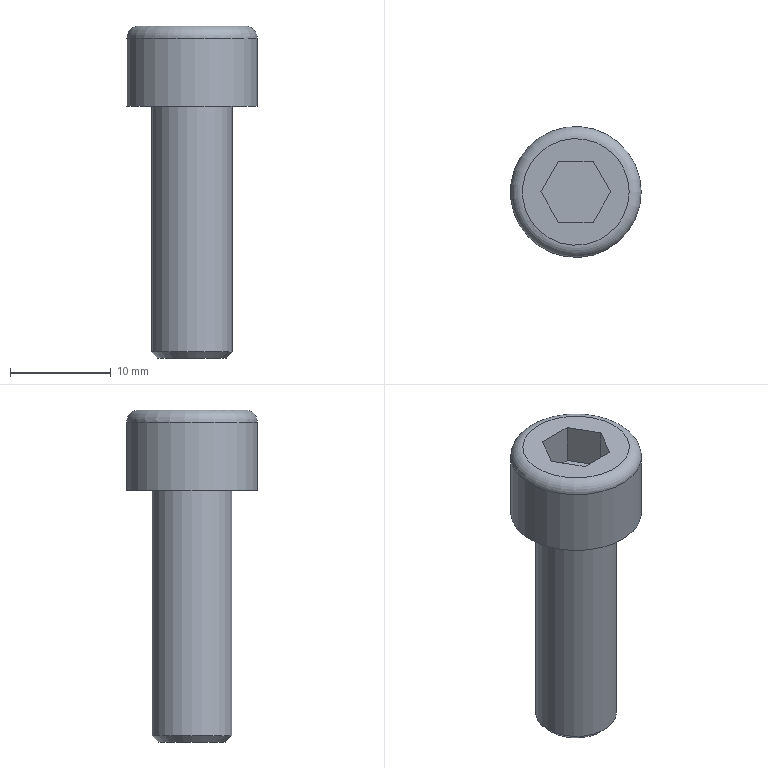Part | STEP file | solid 90 | 1 solid | 14 faces | box 13 x 13 x 33 mm | volume 2177 mm3 | plane 10 | cylinder 2 | torus 1 | cone 1 | commonest cylinder face diameters 8 x1 13 x1